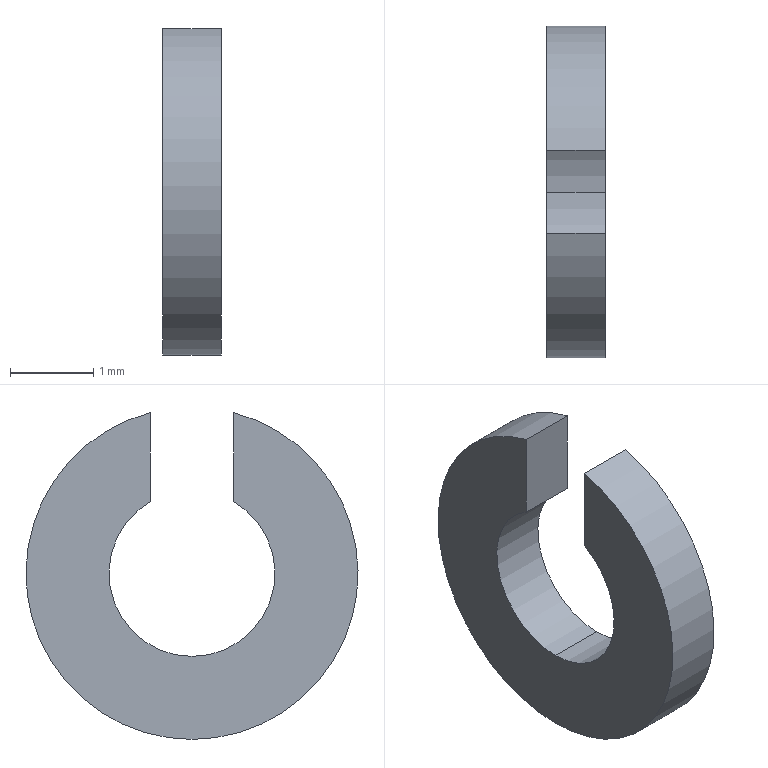Part | STEP file | 0232_Z_SCBJ2-5_2 | 1 solid | 8 faces | box 0.7 x 4 x 3.936 mm | volume 5.882 mm3 | cylinder 4 | plane 4 | commonest cylinder face diameters 2 x2 4 x2
STEP:
#1=CARTESIAN_POINT('',(0.,0.,0.));
#2=DIRECTION('',(0.,0.,1.));
#3=DIRECTION('',(1.,0.,0.));
#4=AXIS2_PLACEMENT_3D('',#1,#2,#3);
#5=CARTESIAN_POINT('',(0.,0.5,0.866));
#6=VERTEX_POINT('',#5);
#7=CARTESIAN_POINT('',(0.7,0.5,0.866));
#8=VERTEX_POINT('',#7);
#9=CARTESIAN_POINT('',(4.35,0.5,0.866));
#10=DIRECTION('',(1.,0.,0.));
#11=VECTOR('',#10,1.);
#12=LINE('',#9,#11);
#13=CARTESIAN_POINT('',(4.35,0.,0.));
#14=DIRECTION('',(1.,0.,0.));
#15=DIRECTION('',(0.,0.,-1.));
#16=AXIS2_PLACEMENT_3D('',#13,#14,#15);
#17=CYLINDRICAL_SURFACE('',#16,1.);
#18=CARTESIAN_POINT('',(2.618,0.));
#19=DIRECTION('',(0.,1.));
#20=VECTOR('',#19,1.);
#21=LINE('',#18,#20);
#22=(GEOMETRIC_REPRESENTATION_CONTEXT(2)PARAMETRIC_REPRESENTATION_CONTEXT()REPRESENTATION_CONTEXT('',''));
#23=DEFINITIONAL_REPRESENTATION('',(#21),#22);
#24=PCURVE('',#17,#23);
#25=CARTESIAN_POINT('',(4.35,0.5,0.866));
#26=DIRECTION('',(0.,1.,0.));
#27=DIRECTION('',(0.,0.,1.));
#28=AXIS2_PLACEMENT_3D('',#25,#26,#27);
#29=PLANE('',#28);
#30=CARTESIAN_POINT('',(0.,0.));
#31=DIRECTION('',(0.,1.));
#32=VECTOR('',#31,1.);
#33=LINE('',#30,#32);
#34=(GEOMETRIC_REPRESENTATION_CONTEXT(2)PARAMETRIC_REPRESENTATION_CONTEXT()REPRESENTATION_CONTEXT('',''));
#35=DEFINITIONAL_REPRESENTATION('',(#33),#34);
#36=PCURVE('',#29,#35);
#37=SURFACE_CURVE('',#12,(#24,#36),.PCURVE_S1.);
#38=EDGE_CURVE('',#6,#8,#37,.T.);
#39=ORIENTED_EDGE('',*,*,#38,.T.);
#40=CARTESIAN_POINT('',(0.7,0.,-1.));
#41=VERTEX_POINT('',#40);
#42=CARTESIAN_POINT('',(0.7,0.,0.));
#43=DIRECTION('',(-1.,0.,0.));
#44=DIRECTION('',(0.,0.,-1.));
#45=AXIS2_PLACEMENT_3D('',#42,#43,#44);
#46=CIRCLE('',#45,1.);
#47=CARTESIAN_POINT('',(6.283,-3.65));
#48=DIRECTION('',(-1.,0.));
#49=VECTOR('',#48,1.);
#50=LINE('',#47,#49);
#51=(GEOMETRIC_REPRESENTATION_CONTEXT(2)PARAMETRIC_REPRESENTATION_CONTEXT()REPRESENTATION_CONTEXT('',''));
#52=DEFINITIONAL_REPRESENTATION('',(#50),#51);
#53=PCURVE('',#17,#52);
#54=CARTESIAN_POINT('',(0.7,1.,0.));
#55=DIRECTION('',(1.,0.,0.));
#56=DIRECTION('',(0.,0.,-1.));
#57=AXIS2_PLACEMENT_3D('',#54,#55,#56);
#58=PLANE('',#57);
#59=CARTESIAN_POINT('',(1.,-1.));
#60=CARTESIAN_POINT('',(1.,-2.732));
#61=CARTESIAN_POINT('',(-0.5,-1.866));
#62=CARTESIAN_POINT('',(-2.,-1.));
#63=CARTESIAN_POINT('',(-0.5,-0.134));
#64=CARTESIAN_POINT('',(1.,0.7321));
#65=CARTESIAN_POINT('',(1.,-1.));
#66=(BOUNDED_CURVE()B_SPLINE_CURVE(2,(#59,#60,#61,#62,#63,#64,#65),.UNSPECIFIED.,.T.,.F.)B_SPLINE_CURVE_WITH_KNOTS((1,2,2,2,2,1),(-2.094,0.,2.094,4.189,6.283,8.378),.UNSPECIFIED.)CURVE()GEOMETRIC_REPRESENTATION_ITEM()RATIONAL_B_SPLINE_CURVE((1.,0.5,1.,0.5,1.,0.5,1.))REPRESENTATION_ITEM(''));
#67=(GEOMETRIC_REPRESENTATION_CONTEXT(2)PARAMETRIC_REPRESENTATION_CONTEXT()REPRESENTATION_CONTEXT('',''));
#68=DEFINITIONAL_REPRESENTATION('',(#66),#67);
#69=PCURVE('',#58,#68);
#70=SURFACE_CURVE('',#46,(#53,#69),.PCURVE_S1.);
#71=EDGE_CURVE('',#8,#41,#70,.T.);
#72=ORIENTED_EDGE('',*,*,#71,.T.);
#73=CARTESIAN_POINT('',(0.,0.,-1.));
#74=VERTEX_POINT('',#73);
#75=CARTESIAN_POINT('',(4.35,0.,-1.));
#76=DIRECTION('',(1.,0.,0.));
#77=VECTOR('',#76,1.);
#78=LINE('',#75,#77);
#79=CARTESIAN_POINT('',(0.,0.));
#80=DIRECTION('',(0.,1.));
#81=VECTOR('',#80,1.);
#82=LINE('',#79,#81);
#83=(GEOMETRIC_REPRESENTATION_CONTEXT(2)PARAMETRIC_REPRESENTATION_CONTEXT()REPRESENTATION_CONTEXT('',''));
#84=DEFINITIONAL_REPRESENTATION('',(#82),#83);
#85=PCURVE('',#17,#84);
#86=CARTESIAN_POINT('',(4.35,0.,0.));
#87=DIRECTION('',(1.,0.,0.));
#88=DIRECTION('',(0.,0.,-1.));
#89=AXIS2_PLACEMENT_3D('',#86,#87,#88);
#90=CYLINDRICAL_SURFACE('',#89,1.);
#91=CARTESIAN_POINT('',(6.283,0.));
#92=DIRECTION('',(0.,1.));
#93=VECTOR('',#92,1.);
#94=LINE('',#91,#93);
#95=(GEOMETRIC_REPRESENTATION_CONTEXT(2)PARAMETRIC_REPRESENTATION_CONTEXT()REPRESENTATION_CONTEXT('',''));
#96=DEFINITIONAL_REPRESENTATION('',(#94),#95);
#97=PCURVE('',#90,#96);
#98=SURFACE_CURVE('',#78,(#85,#97),.PCURVE_S1.);
#99=EDGE_CURVE('',#74,#41,#98,.T.);
#100=ORIENTED_EDGE('',*,*,#99,.F.);
#101=CARTESIAN_POINT('',(0.,0.,0.));
#102=DIRECTION('',(1.,0.,0.));
#103=DIRECTION('',(0.,0.,-1.));
#104=AXIS2_PLACEMENT_3D('',#101,#102,#103);
#105=CIRCLE('',#104,1.);
#106=CARTESIAN_POINT('',(0.,-4.35));
#107=DIRECTION('',(1.,0.));
#108=VECTOR('',#107,1.);
#109=LINE('',#106,#108);
#110=(GEOMETRIC_REPRESENTATION_CONTEXT(2)PARAMETRIC_REPRESENTATION_CONTEXT()REPRESENTATION_CONTEXT('',''));
#111=DEFINITIONAL_REPRESENTATION('',(#109),#110);
#112=PCURVE('',#17,#111);
#113=CARTESIAN_POINT('',(0.,1.,0.));
#114=DIRECTION('',(-1.,0.,0.));
#115=DIRECTION('',(0.,0.,1.));
#116=AXIS2_PLACEMENT_3D('',#113,#114,#115);
#117=PLANE('',#116);
#118=CARTESIAN_POINT('',(-1.,-1.));
#119=CARTESIAN_POINT('',(-1.,0.7321));
#120=CARTESIAN_POINT('',(0.5,-0.134));
#121=CARTESIAN_POINT('',(2.,-1.));
#122=CARTESIAN_POINT('',(0.5,-1.866));
#123=CARTESIAN_POINT('',(-1.,-2.732));
#124=CARTESIAN_POINT('',(-1.,-1.));
#125=(BOUNDED_CURVE()B_SPLINE_CURVE(2,(#118,#119,#120,#121,#122,#123,#124),.UNSPECIFIED.,.T.,.F.)B_SPLINE_CURVE_WITH_KNOTS((1,2,2,2,2,1),(-2.094,0.,2.094,4.189,6.283,8.378),.UNSPECIFIED.)CURVE()GEOMETRIC_REPRESENTATION_ITEM()RATIONAL_B_SPLINE_CURVE((1.,0.5,1.,0.5,1.,0.5,1.))REPRESENTATION_ITEM(''));
#126=(GEOMETRIC_REPRESENTATION_CONTEXT(2)PARAMETRIC_REPRESENTATION_CONTEXT()REPRESENTATION_CONTEXT('',''));
#127=DEFINITIONAL_REPRESENTATION('',(#125),#126);
#128=PCURVE('',#117,#127);
#129=SURFACE_CURVE('',#105,(#112,#128),.PCURVE_S1.);
#130=EDGE_CURVE('',#74,#6,#129,.T.);
#131=ORIENTED_EDGE('',*,*,#130,.T.);
#132=EDGE_LOOP('',(#39,#72,#100,#131));
#133=FACE_BOUND('',#132,.F.);
#134=ADVANCED_FACE('',(#133),#17,.F.);
#135=CARTESIAN_POINT('',(0.,0.,-2.));
#136=VERTEX_POINT('',#135);
#137=CARTESIAN_POINT('',(0.,-0.5,1.936));
#138=VERTEX_POINT('',#137);
#139=CARTESIAN_POINT('',(0.,0.,0.));
#140=DIRECTION('',(-1.,0.,0.));
#141=DIRECTION('',(0.,0.,-1.));
#142=AXIS2_PLACEMENT_3D('',#139,#140,#141);
#143=CIRCLE('',#142,2.);
#144=CARTESIAN_POINT('',(0.35,0.,0.));
#145=DIRECTION('',(1.,0.,0.));
#146=DIRECTION('',(0.,0.,-1.));
#147=AXIS2_PLACEMENT_3D('',#144,#145,#146);
#148=CYLINDRICAL_SURFACE('',#147,2.);
#149=CARTESIAN_POINT('',(6.283,-0.35));
#150=DIRECTION('',(-1.,0.));
#151=VECTOR('',#150,1.);
#152=LINE('',#149,#151);
#153=(GEOMETRIC_REPRESENTATION_CONTEXT(2)PARAMETRIC_REPRESENTATION_CONTEXT()REPRESENTATION_CONTEXT('',''));
#154=DEFINITIONAL_REPRESENTATION('',(#152),#153);
#155=PCURVE('',#148,#154);
#156=CARTESIAN_POINT('',(0.,-1.));
#157=DIRECTION('',(-1.,0.));
#158=AXIS2_PLACEMENT_2D('',#156,#157);
#159=CIRCLE('',#158,2.);
#160=(GEOMETRIC_REPRESENTATION_CONTEXT(2)PARAMETRIC_REPRESENTATION_CONTEXT()REPRESENTATION_CONTEXT('',''));
#161=DEFINITIONAL_REPRESENTATION('',(#159),#160);
#162=PCURVE('',#117,#161);
#163=SURFACE_CURVE('',#143,(#155,#162),.PCURVE_S1.);
#164=EDGE_CURVE('',#136,#138,#163,.T.);
#165=ORIENTED_EDGE('',*,*,#164,.F.);
#166=CARTESIAN_POINT('',(0.7,0.,-2.));
#167=VERTEX_POINT('',#166);
#168=CARTESIAN_POINT('',(0.35,0.,-2.));
#169=DIRECTION('',(1.,0.,0.));
#170=VECTOR('',#169,1.);
#171=LINE('',#168,#170);
#172=CARTESIAN_POINT('',(6.283,0.));
#173=DIRECTION('',(0.,1.));
#174=VECTOR('',#173,1.);
#175=LINE('',#172,#174);
#176=(GEOMETRIC_REPRESENTATION_CONTEXT(2)PARAMETRIC_REPRESENTATION_CONTEXT()REPRESENTATION_CONTEXT('',''));
#177=DEFINITIONAL_REPRESENTATION('',(#175),#176);
#178=PCURVE('',#148,#177);
#179=CARTESIAN_POINT('',(0.35,0.,0.));
#180=DIRECTION('',(1.,0.,0.));
#181=DIRECTION('',(0.,0.,-1.));
#182=AXIS2_PLACEMENT_3D('',#179,#180,#181);
#183=CYLINDRICAL_SURFACE('',#182,2.);
#184=CARTESIAN_POINT('',(0.,0.));
#185=DIRECTION('',(0.,1.));
#186=VECTOR('',#185,1.);
#187=LINE('',#184,#186);
#188=(GEOMETRIC_REPRESENTATION_CONTEXT(2)PARAMETRIC_REPRESENTATION_CONTEXT()REPRESENTATION_CONTEXT('',''));
#189=DEFINITIONAL_REPRESENTATION('',(#187),#188);
#190=PCURVE('',#183,#189);
#191=SURFACE_CURVE('',#171,(#178,#190),.PCURVE_S1.);
#192=EDGE_CURVE('',#136,#167,#191,.T.);
#193=ORIENTED_EDGE('',*,*,#192,.T.);
#194=CARTESIAN_POINT('',(0.7,-0.5,1.936));
#195=VERTEX_POINT('',#194);
#196=CARTESIAN_POINT('',(0.7,0.,0.));
#197=DIRECTION('',(-1.,0.,0.));
#198=DIRECTION('',(0.,0.,-1.));
#199=AXIS2_PLACEMENT_3D('',#196,#197,#198);
#200=CIRCLE('',#199,2.);
#201=CARTESIAN_POINT('',(6.283,0.35));
#202=DIRECTION('',(-1.,0.));
#203=VECTOR('',#202,1.);
#204=LINE('',#201,#203);
#205=(GEOMETRIC_REPRESENTATION_CONTEXT(2)PARAMETRIC_REPRESENTATION_CONTEXT()REPRESENTATION_CONTEXT('',''));
#206=DEFINITIONAL_REPRESENTATION('',(#204),#205);
#207=PCURVE('',#148,#206);
#208=CARTESIAN_POINT('',(2.,-1.));
#209=CARTESIAN_POINT('',(2.,-4.464));
#210=CARTESIAN_POINT('',(-1.,-2.732));
#211=CARTESIAN_POINT('',(-4.,-1.));
#212=CARTESIAN_POINT('',(-1.,0.7321));
#213=CARTESIAN_POINT('',(2.,2.464));
#214=CARTESIAN_POINT('',(2.,-1.));
#215=(BOUNDED_CURVE()B_SPLINE_CURVE(2,(#208,#209,#210,#211,#212,#213,#214),.UNSPECIFIED.,.T.,.F.)B_SPLINE_CURVE_WITH_KNOTS((1,2,2,2,2,1),(-2.094,0.,2.094,4.189,6.283,8.378),.UNSPECIFIED.)CURVE()GEOMETRIC_REPRESENTATION_ITEM()RATIONAL_B_SPLINE_CURVE((1.,0.5,1.,0.5,1.,0.5,1.))REPRESENTATION_ITEM(''));
#216=(GEOMETRIC_REPRESENTATION_CONTEXT(2)PARAMETRIC_REPRESENTATION_CONTEXT()REPRESENTATION_CONTEXT('',''));
#217=DEFINITIONAL_REPRESENTATION('',(#215),#216);
#218=PCURVE('',#58,#217);
#219=SURFACE_CURVE('',#200,(#207,#218),.PCURVE_S1.);
#220=EDGE_CURVE('',#167,#195,#219,.T.);
#221=ORIENTED_EDGE('',*,*,#220,.T.);
#222=CARTESIAN_POINT('',(4.35,-0.5,1.936));
#223=DIRECTION('',(-1.,0.,0.));
#224=VECTOR('',#223,1.);
#225=LINE('',#222,#224);
#226=CARTESIAN_POINT('',(3.394,4.));
#227=DIRECTION('',(0.,-1.));
#228=VECTOR('',#227,1.);
#229=LINE('',#226,#228);
#230=(GEOMETRIC_REPRESENTATION_CONTEXT(2)PARAMETRIC_REPRESENTATION_CONTEXT()REPRESENTATION_CONTEXT('',''));
#231=DEFINITIONAL_REPRESENTATION('',(#229),#230);
#232=PCURVE('',#148,#231);
#233=CARTESIAN_POINT('',(4.35,-0.5,2.));
#234=DIRECTION('',(0.,-1.,0.));
#235=DIRECTION('',(0.,0.,-1.));
#236=AXIS2_PLACEMENT_3D('',#233,#234,#235);
#237=PLANE('',#236);
#238=CARTESIAN_POINT('',(0.06351,0.));
#239=DIRECTION('',(0.,-1.));
#240=VECTOR('',#239,1.);
#241=LINE('',#238,#240);
#242=(GEOMETRIC_REPRESENTATION_CONTEXT(2)PARAMETRIC_REPRESENTATION_CONTEXT()REPRESENTATION_CONTEXT('',''));
#243=DEFINITIONAL_REPRESENTATION('',(#241),#242);
#244=PCURVE('',#237,#243);
#245=SURFACE_CURVE('',#225,(#232,#244),.PCURVE_S1.);
#246=EDGE_CURVE('',#195,#138,#245,.T.);
#247=ORIENTED_EDGE('',*,*,#246,.T.);
#248=EDGE_LOOP('',(#165,#193,#221,#247));
#249=FACE_BOUND('',#248,.T.);
#250=ADVANCED_FACE('',(#249),#148,.T.);
#251=CARTESIAN_POINT('',(0.,-0.5,0.866));
#252=VERTEX_POINT('',#251);
#253=CARTESIAN_POINT('',(0.,0.,0.));
#254=DIRECTION('',(1.,0.,0.));
#255=DIRECTION('',(0.,0.,-1.));
#256=AXIS2_PLACEMENT_3D('',#253,#254,#255);
#257=CIRCLE('',#256,1.);
#258=CARTESIAN_POINT('',(-1.,-1.));
#259=CARTESIAN_POINT('',(-1.,0.7321));
#260=CARTESIAN_POINT('',(0.5,-0.134));
#261=CARTESIAN_POINT('',(2.,-1.));
#262=CARTESIAN_POINT('',(0.5,-1.866));
#263=CARTESIAN_POINT('',(-1.,-2.732));
#264=CARTESIAN_POINT('',(-1.,-1.));
#265=(BOUNDED_CURVE()B_SPLINE_CURVE(2,(#258,#259,#260,#261,#262,#263,#264),.UNSPECIFIED.,.T.,.F.)B_SPLINE_CURVE_WITH_KNOTS((1,2,2,2,2,1),(-2.094,0.,2.094,4.189,6.283,8.378),.UNSPECIFIED.)CURVE()GEOMETRIC_REPRESENTATION_ITEM()RATIONAL_B_SPLINE_CURVE((1.,0.5,1.,0.5,1.,0.5,1.))REPRESENTATION_ITEM(''));
#266=(GEOMETRIC_REPRESENTATION_CONTEXT(2)PARAMETRIC_REPRESENTATION_CONTEXT()REPRESENTATION_CONTEXT('',''));
#267=DEFINITIONAL_REPRESENTATION('',(#265),#266);
#268=PCURVE('',#117,#267);
#269=CARTESIAN_POINT('',(0.,-4.35));
#270=DIRECTION('',(1.,0.));
#271=VECTOR('',#270,1.);
#272=LINE('',#269,#271);
#273=(GEOMETRIC_REPRESENTATION_CONTEXT(2)PARAMETRIC_REPRESENTATION_CONTEXT()REPRESENTATION_CONTEXT('',''));
#274=DEFINITIONAL_REPRESENTATION('',(#272),#273);
#275=PCURVE('',#90,#274);
#276=SURFACE_CURVE('',#257,(#268,#275),.PCURVE_S1.);
#277=EDGE_CURVE('',#252,#74,#276,.T.);
#278=ORIENTED_EDGE('',*,*,#277,.T.);
#279=ORIENTED_EDGE('',*,*,#130,.T.);
#280=CARTESIAN_POINT('',(0.,0.5,1.936));
#281=VERTEX_POINT('',#280);
#282=CARTESIAN_POINT('',(0.,0.5,0.));
#283=DIRECTION('',(0.,0.,1.));
#284=VECTOR('',#283,1.);
#285=LINE('',#282,#284);
#286=CARTESIAN_POINT('',(0.,-0.5));
#287=DIRECTION('',(1.,0.));
#288=VECTOR('',#287,1.);
#289=LINE('',#286,#288);
#290=(GEOMETRIC_REPRESENTATION_CONTEXT(2)PARAMETRIC_REPRESENTATION_CONTEXT()REPRESENTATION_CONTEXT('',''));
#291=DEFINITIONAL_REPRESENTATION('',(#289),#290);
#292=PCURVE('',#117,#291);
#293=CARTESIAN_POINT('',(-0.866,-4.35));
#294=DIRECTION('',(1.,0.));
#295=VECTOR('',#294,1.);
#296=LINE('',#293,#295);
#297=(GEOMETRIC_REPRESENTATION_CONTEXT(2)PARAMETRIC_REPRESENTATION_CONTEXT()REPRESENTATION_CONTEXT('',''));
#298=DEFINITIONAL_REPRESENTATION('',(#296),#297);
#299=PCURVE('',#29,#298);
#300=SURFACE_CURVE('',#285,(#292,#299),.PCURVE_S1.);
#301=EDGE_CURVE('',#6,#281,#300,.T.);
#302=ORIENTED_EDGE('',*,*,#301,.T.);
#303=CARTESIAN_POINT('',(0.,0.,0.));
#304=DIRECTION('',(-1.,0.,0.));
#305=DIRECTION('',(0.,0.,-1.));
#306=AXIS2_PLACEMENT_3D('',#303,#304,#305);
#307=CIRCLE('',#306,2.);
#308=CARTESIAN_POINT('',(0.,-1.));
#309=DIRECTION('',(-1.,0.));
#310=AXIS2_PLACEMENT_2D('',#308,#309);
#311=CIRCLE('',#310,2.);
#312=(GEOMETRIC_REPRESENTATION_CONTEXT(2)PARAMETRIC_REPRESENTATION_CONTEXT()REPRESENTATION_CONTEXT('',''));
#313=DEFINITIONAL_REPRESENTATION('',(#311),#312);
#314=PCURVE('',#117,#313);
#315=CARTESIAN_POINT('',(6.283,-0.35));
#316=DIRECTION('',(-1.,0.));
#317=VECTOR('',#316,1.);
#318=LINE('',#315,#317);
#319=(GEOMETRIC_REPRESENTATION_CONTEXT(2)PARAMETRIC_REPRESENTATION_CONTEXT()REPRESENTATION_CONTEXT('',''));
#320=DEFINITIONAL_REPRESENTATION('',(#318),#319);
#321=PCURVE('',#183,#320);
#322=SURFACE_CURVE('',#307,(#314,#321),.PCURVE_S1.);
#323=EDGE_CURVE('',#281,#136,#322,.T.);
#324=ORIENTED_EDGE('',*,*,#323,.T.);
#325=ORIENTED_EDGE('',*,*,#164,.T.);
#326=CARTESIAN_POINT('',(0.,-0.5,0.));
#327=DIRECTION('',(0.,0.,-1.));
#328=VECTOR('',#327,1.);
#329=LINE('',#326,#328);
#330=CARTESIAN_POINT('',(0.,-1.5));
#331=DIRECTION('',(-1.,0.));
#332=VECTOR('',#331,1.);
#333=LINE('',#330,#332);
#334=(GEOMETRIC_REPRESENTATION_CONTEXT(2)PARAMETRIC_REPRESENTATION_CONTEXT()REPRESENTATION_CONTEXT('',''));
#335=DEFINITIONAL_REPRESENTATION('',(#333),#334);
#336=PCURVE('',#117,#335);
#337=CARTESIAN_POINT('',(2.,-4.35));
#338=DIRECTION('',(1.,0.));
#339=VECTOR('',#338,1.);
#340=LINE('',#337,#339);
#341=(GEOMETRIC_REPRESENTATION_CONTEXT(2)PARAMETRIC_REPRESENTATION_CONTEXT()REPRESENTATION_CONTEXT('',''));
#342=DEFINITIONAL_REPRESENTATION('',(#340),#341);
#343=PCURVE('',#237,#342);
#344=SURFACE_CURVE('',#329,(#336,#343),.PCURVE_S1.);
#345=EDGE_CURVE('',#138,#252,#344,.T.);
#346=ORIENTED_EDGE('',*,*,#345,.T.);
#347=EDGE_LOOP('',(#278,#279,#302,#324,#325,#346));
#348=FACE_BOUND('',#347,.T.);
#349=ADVANCED_FACE('',(#348),#117,.T.);
#350=CARTESIAN_POINT('',(0.7,-0.5,0.866));
#351=VERTEX_POINT('',#350);
#352=CARTESIAN_POINT('',(0.7,0.,0.));
#353=DIRECTION('',(-1.,0.,0.));
#354=DIRECTION('',(0.,0.,-1.));
#355=AXIS2_PLACEMENT_3D('',#352,#353,#354);
#356=CIRCLE('',#355,1.);
#357=CARTESIAN_POINT('',(6.283,-3.65));
#358=DIRECTION('',(-1.,0.));
#359=VECTOR('',#358,1.);
#360=LINE('',#357,#359);
#361=(GEOMETRIC_REPRESENTATION_CONTEXT(2)PARAMETRIC_REPRESENTATION_CONTEXT()REPRESENTATION_CONTEXT('',''));
#362=DEFINITIONAL_REPRESENTATION('',(#360),#361);
#363=PCURVE('',#90,#362);
#364=CARTESIAN_POINT('',(1.,-1.));
#365=CARTESIAN_POINT('',(1.,-2.732));
#366=CARTESIAN_POINT('',(-0.5,-1.866));
#367=CARTESIAN_POINT('',(-2.,-1.));
#368=CARTESIAN_POINT('',(-0.5,-0.134));
#369=CARTESIAN_POINT('',(1.,0.7321));
#370=CARTESIAN_POINT('',(1.,-1.));
#371=(BOUNDED_CURVE()B_SPLINE_CURVE(2,(#364,#365,#366,#367,#368,#369,#370),.UNSPECIFIED.,.T.,.F.)B_SPLINE_CURVE_WITH_KNOTS((1,2,2,2,2,1),(-2.094,0.,2.094,4.189,6.283,8.378),.UNSPECIFIED.)CURVE()GEOMETRIC_REPRESENTATION_ITEM()RATIONAL_B_SPLINE_CURVE((1.,0.5,1.,0.5,1.,0.5,1.))REPRESENTATION_ITEM(''));
#372=(GEOMETRIC_REPRESENTATION_CONTEXT(2)PARAMETRIC_REPRESENTATION_CONTEXT()REPRESENTATION_CONTEXT('',''));
#373=DEFINITIONAL_REPRESENTATION('',(#371),#372);
#374=PCURVE('',#58,#373);
#375=SURFACE_CURVE('',#356,(#363,#374),.PCURVE_S1.);
#376=EDGE_CURVE('',#41,#351,#375,.T.);
#377=ORIENTED_EDGE('',*,*,#376,.T.);
#378=CARTESIAN_POINT('',(4.35,-0.5,0.866));
#379=DIRECTION('',(-1.,0.,0.));
#380=VECTOR('',#379,1.);
#381=LINE('',#378,#380);
#382=CARTESIAN_POINT('',(3.665,0.));
#383=DIRECTION('',(0.,-1.));
#384=VECTOR('',#383,1.);
#385=LINE('',#382,#384);
#386=(GEOMETRIC_REPRESENTATION_CONTEXT(2)PARAMETRIC_REPRESENTATION_CONTEXT()REPRESENTATION_CONTEXT('',''));
#387=DEFINITIONAL_REPRESENTATION('',(#385),#386);
#388=PCURVE('',#90,#387);
#389=CARTESIAN_POINT('',(1.134,0.));
#390=DIRECTION('',(0.,-1.));
#391=VECTOR('',#390,1.);
#392=LINE('',#389,#391);
#393=(GEOMETRIC_REPRESENTATION_CONTEXT(2)PARAMETRIC_REPRESENTATION_CONTEXT()REPRESENTATION_CONTEXT('',''));
#394=DEFINITIONAL_REPRESENTATION('',(#392),#393);
#395=PCURVE('',#237,#394);
#396=SURFACE_CURVE('',#381,(#388,#395),.PCURVE_S1.);
#397=EDGE_CURVE('',#351,#252,#396,.T.);
#398=ORIENTED_EDGE('',*,*,#397,.T.);
#399=ORIENTED_EDGE('',*,*,#277,.T.);
#400=ORIENTED_EDGE('',*,*,#99,.T.);
#401=EDGE_LOOP('',(#377,#398,#399,#400));
#402=FACE_BOUND('',#401,.F.);
#403=ADVANCED_FACE('',(#402),#90,.F.);
#404=ORIENTED_EDGE('',*,*,#397,.T.);
#405=ORIENTED_EDGE('',*,*,#345,.F.);
#406=ORIENTED_EDGE('',*,*,#246,.F.);
#407=CARTESIAN_POINT('',(0.7,-0.5,2.));
#408=DIRECTION('',(0.,0.,1.));
#409=VECTOR('',#408,1.);
#410=LINE('',#407,#409);
#411=CARTESIAN_POINT('',(0.,-3.65));
#412=DIRECTION('',(-1.,0.));
#413=VECTOR('',#412,1.);
#414=LINE('',#411,#413);
#415=(GEOMETRIC_REPRESENTATION_CONTEXT(2)PARAMETRIC_REPRESENTATION_CONTEXT()REPRESENTATION_CONTEXT('',''));
#416=DEFINITIONAL_REPRESENTATION('',(#414),#415);
#417=PCURVE('',#237,#416);
#418=CARTESIAN_POINT('',(-2.,-1.5));
#419=DIRECTION('',(-1.,0.));
#420=VECTOR('',#419,1.);
#421=LINE('',#418,#420);
#422=(GEOMETRIC_REPRESENTATION_CONTEXT(2)PARAMETRIC_REPRESENTATION_CONTEXT()REPRESENTATION_CONTEXT('',''));
#423=DEFINITIONAL_REPRESENTATION('',(#421),#422);
#424=PCURVE('',#58,#423);
#425=SURFACE_CURVE('',#410,(#417,#424),.PCURVE_S1.);
#426=EDGE_CURVE('',#351,#195,#425,.T.);
#427=ORIENTED_EDGE('',*,*,#426,.F.);
#428=EDGE_LOOP('',(#404,#405,#406,#427));
#429=FACE_BOUND('',#428,.T.);
#430=ADVANCED_FACE('',(#429),#237,.F.);
#431=ORIENTED_EDGE('',*,*,#192,.F.);
#432=ORIENTED_EDGE('',*,*,#323,.F.);
#433=CARTESIAN_POINT('',(0.7,0.5,1.936));
#434=VERTEX_POINT('',#433);
#435=CARTESIAN_POINT('',(0.35,0.5,1.936));
#436=DIRECTION('',(1.,0.,0.));
#437=VECTOR('',#436,1.);
#438=LINE('',#435,#437);
#439=CARTESIAN_POINT('',(2.889,0.));
#440=DIRECTION('',(0.,1.));
#441=VECTOR('',#440,1.);
#442=LINE('',#439,#441);
#443=(GEOMETRIC_REPRESENTATION_CONTEXT(2)PARAMETRIC_REPRESENTATION_CONTEXT()REPRESENTATION_CONTEXT('',''));
#444=DEFINITIONAL_REPRESENTATION('',(#442),#443);
#445=PCURVE('',#183,#444);
#446=CARTESIAN_POINT('',(1.07,-4.));
#447=DIRECTION('',(0.,1.));
#448=VECTOR('',#447,1.);
#449=LINE('',#446,#448);
#450=(GEOMETRIC_REPRESENTATION_CONTEXT(2)PARAMETRIC_REPRESENTATION_CONTEXT()REPRESENTATION_CONTEXT('',''));
#451=DEFINITIONAL_REPRESENTATION('',(#449),#450);
#452=PCURVE('',#29,#451);
#453=SURFACE_CURVE('',#438,(#445,#452),.PCURVE_S1.);
#454=EDGE_CURVE('',#281,#434,#453,.T.);
#455=ORIENTED_EDGE('',*,*,#454,.T.);
#456=CARTESIAN_POINT('',(0.7,0.,0.));
#457=DIRECTION('',(-1.,0.,0.));
#458=DIRECTION('',(0.,0.,-1.));
#459=AXIS2_PLACEMENT_3D('',#456,#457,#458);
#460=CIRCLE('',#459,2.);
#461=CARTESIAN_POINT('',(6.283,0.35));
#462=DIRECTION('',(-1.,0.));
#463=VECTOR('',#462,1.);
#464=LINE('',#461,#463);
#465=(GEOMETRIC_REPRESENTATION_CONTEXT(2)PARAMETRIC_REPRESENTATION_CONTEXT()REPRESENTATION_CONTEXT('',''));
#466=DEFINITIONAL_REPRESENTATION('',(#464),#465);
#467=PCURVE('',#183,#466);
#468=CARTESIAN_POINT('',(2.,-1.));
#469=CARTESIAN_POINT('',(2.,-4.464));
#470=CARTESIAN_POINT('',(-1.,-2.732));
#471=CARTESIAN_POINT('',(-4.,-1.));
#472=CARTESIAN_POINT('',(-1.,0.7321));
#473=CARTESIAN_POINT('',(2.,2.464));
#474=CARTESIAN_POINT('',(2.,-1.));
#475=(BOUNDED_CURVE()B_SPLINE_CURVE(2,(#468,#469,#470,#471,#472,#473,#474),.UNSPECIFIED.,.T.,.F.)B_SPLINE_CURVE_WITH_KNOTS((1,2,2,2,2,1),(-2.094,0.,2.094,4.189,6.283,8.378),.UNSPECIFIED.)CURVE()GEOMETRIC_REPRESENTATION_ITEM()RATIONAL_B_SPLINE_CURVE((1.,0.5,1.,0.5,1.,0.5,1.))REPRESENTATION_ITEM(''));
#476=(GEOMETRIC_REPRESENTATION_CONTEXT(2)PARAMETRIC_REPRESENTATION_CONTEXT()REPRESENTATION_CONTEXT('',''));
#477=DEFINITIONAL_REPRESENTATION('',(#475),#476);
#478=PCURVE('',#58,#477);
#479=SURFACE_CURVE('',#460,(#467,#478),.PCURVE_S1.);
#480=EDGE_CURVE('',#434,#167,#479,.T.);
#481=ORIENTED_EDGE('',*,*,#480,.T.);
#482=EDGE_LOOP('',(#431,#432,#455,#481));
#483=FACE_BOUND('',#482,.T.);
#484=ADVANCED_FACE('',(#483),#183,.T.);
#485=ORIENTED_EDGE('',*,*,#454,.F.);
#486=ORIENTED_EDGE('',*,*,#301,.F.);
#487=ORIENTED_EDGE('',*,*,#38,.T.);
#488=CARTESIAN_POINT('',(0.7,0.5,0.866));
#489=DIRECTION('',(0.,0.,-1.));
#490=VECTOR('',#489,1.);
#491=LINE('',#488,#490);
#492=CARTESIAN_POINT('',(0.,-3.65));
#493=DIRECTION('',(-1.,0.));
#494=VECTOR('',#493,1.);
#495=LINE('',#492,#494);
#496=(GEOMETRIC_REPRESENTATION_CONTEXT(2)PARAMETRIC_REPRESENTATION_CONTEXT()REPRESENTATION_CONTEXT('',''));
#497=DEFINITIONAL_REPRESENTATION('',(#495),#496);
#498=PCURVE('',#29,#497);
#499=CARTESIAN_POINT('',(-0.866,-0.5));
#500=DIRECTION('',(1.,0.));
#501=VECTOR('',#500,1.);
#502=LINE('',#499,#501);
#503=(GEOMETRIC_REPRESENTATION_CONTEXT(2)PARAMETRIC_REPRESENTATION_CONTEXT()REPRESENTATION_CONTEXT('',''));
#504=DEFINITIONAL_REPRESENTATION('',(#502),#503);
#505=PCURVE('',#58,#504);
#506=SURFACE_CURVE('',#491,(#498,#505),.PCURVE_S1.);
#507=EDGE_CURVE('',#434,#8,#506,.T.);
#508=ORIENTED_EDGE('',*,*,#507,.F.);
#509=EDGE_LOOP('',(#485,#486,#487,#508));
#510=FACE_BOUND('',#509,.T.);
#511=ADVANCED_FACE('',(#510),#29,.F.);
#512=ORIENTED_EDGE('',*,*,#480,.F.);
#513=ORIENTED_EDGE('',*,*,#507,.T.);
#514=ORIENTED_EDGE('',*,*,#71,.T.);
#515=ORIENTED_EDGE('',*,*,#376,.T.);
#516=ORIENTED_EDGE('',*,*,#426,.T.);
#517=ORIENTED_EDGE('',*,*,#220,.F.);
#518=EDGE_LOOP('',(#512,#513,#514,#515,#516,#517));
#519=FACE_BOUND('',#518,.T.);
#520=ADVANCED_FACE('',(#519),#58,.T.);
#521=CLOSED_SHELL('',(#134,#250,#349,#403,#430,#484,#511,#520));
#522=MANIFOLD_SOLID_BREP('',#521);
#523=(LENGTH_UNIT()NAMED_UNIT(*)SI_UNIT(.MILLI.,.METRE.));
#524=UNCERTAINTY_MEASURE_WITH_UNIT(LENGTH_MEASURE(0.0000001),#523,'','');
#525=(NAMED_UNIT(*)PLANE_ANGLE_UNIT()SI_UNIT($,.RADIAN.));
#526=(NAMED_UNIT(*)SI_UNIT($,.STERADIAN.)SOLID_ANGLE_UNIT());
#527=(GEOMETRIC_REPRESENTATION_CONTEXT(3)GLOBAL_UNCERTAINTY_ASSIGNED_CONTEXT((#524))GLOBAL_UNIT_ASSIGNED_CONTEXT((#523,#525,#526))REPRESENTATION_CONTEXT('',''));
#528=ADVANCED_BREP_SHAPE_REPRESENTATION('',(#4,#522),#527);